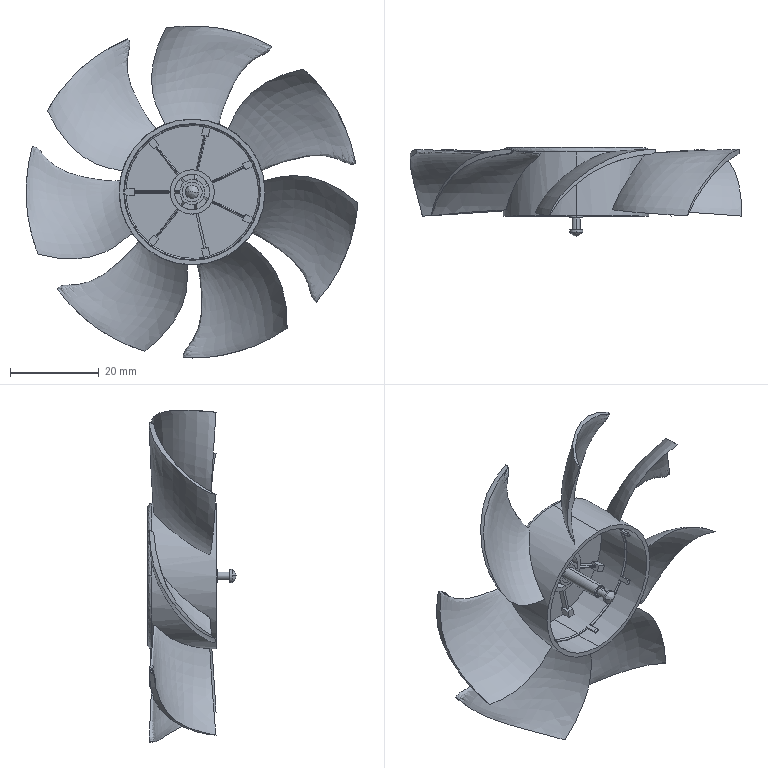Part | STEP file | 8025RYE_3_1 | 1 solid | 195 faces | box 74.924 x 20.1 x 75 mm | volume 5435 mm3 | plane 105 | cylinder 47 | spline 35 | cone 8 | commonest cylinder face diameters 0.4 x12 75 x8 26.1 x7 2.992 x4 1.8 x2 4.5 x2